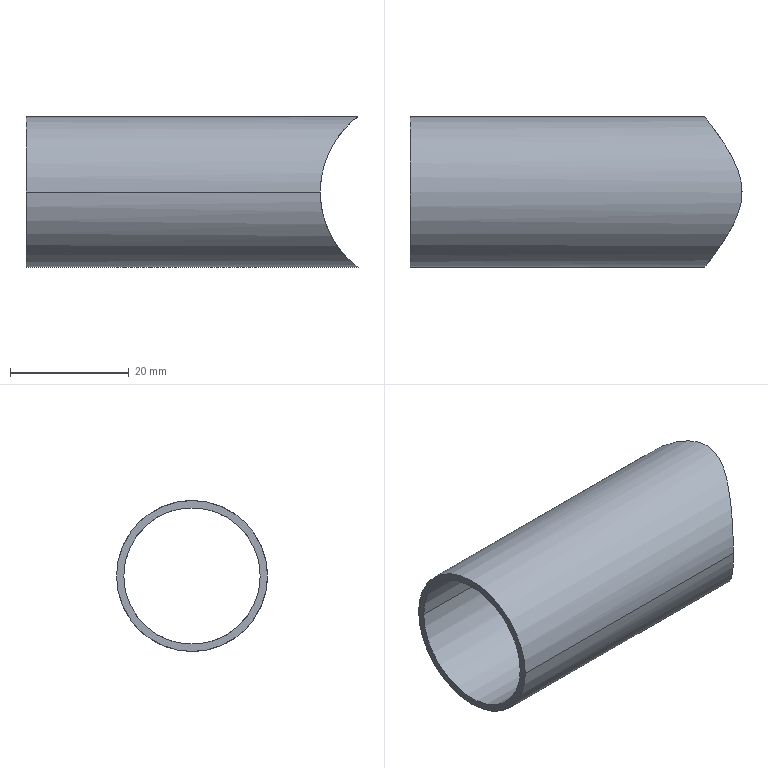Part | NX | features BREP 1 | 1 solid | 6 faces | box 55.88 x 25.4 x 25.4 mm | volume 4831 mm3 | cylinder 5 | plane 1 | commonest cylinder face diameters 22.962 x2 25.4 x2 31.75 x1
STEP:
#1=CARTESIAN_POINT('',(0.,12.7,0.));
#2=VERTEX_POINT('',#1);
#3=CARTESIAN_POINT('',(0.,-12.7,0.));
#4=VERTEX_POINT('',#3);
#5=CARTESIAN_POINT('',(0.,0.,0.));
#6=DIRECTION('',(1.,0.,0.));
#7=DIRECTION('',(0.,1.,0.));
#8=AXIS2_PLACEMENT_3D('',#5,#6,#7);
#9=CIRCLE('',#8,12.7);
#10=EDGE_CURVE('',#2,#4,#9,.T.);
#11=ORIENTED_EDGE('',*,*,#10,.F.);
#12=CARTESIAN_POINT('',(0.,0.,0.));
#13=DIRECTION('',(1.,0.,0.));
#14=DIRECTION('',(0.,-1.,0.));
#15=AXIS2_PLACEMENT_3D('',#12,#13,#14);
#16=CIRCLE('',#15,12.7);
#17=EDGE_CURVE('',#4,#2,#16,.T.);
#18=ORIENTED_EDGE('',*,*,#17,.F.);
#19=EDGE_LOOP('',(#11,#18));
#20=FACE_BOUND('',#19,.T.);
#21=CARTESIAN_POINT('',(0.,11.481,0.));
#22=VERTEX_POINT('',#21);
#23=CARTESIAN_POINT('',(0.,-11.481,0.));
#24=VERTEX_POINT('',#23);
#25=CARTESIAN_POINT('',(0.,0.,0.));
#26=DIRECTION('',(-1.,0.,0.));
#27=DIRECTION('',(0.,1.,0.));
#28=AXIS2_PLACEMENT_3D('',#25,#26,#27);
#29=CIRCLE('',#28,11.481);
#30=EDGE_CURVE('',#22,#24,#29,.T.);
#31=ORIENTED_EDGE('',*,*,#30,.F.);
#32=CARTESIAN_POINT('',(0.,0.,0.));
#33=DIRECTION('',(-1.,0.,0.));
#34=DIRECTION('',(0.,-1.,0.));
#35=AXIS2_PLACEMENT_3D('',#32,#33,#34);
#36=CIRCLE('',#35,11.481);
#37=EDGE_CURVE('',#24,#22,#36,.T.);
#38=ORIENTED_EDGE('',*,*,#37,.F.);
#39=EDGE_LOOP('',(#31,#38));
#40=FACE_BOUND('',#39,.T.);
#41=CARTESIAN_POINT('',(0.,0.,0.));
#42=DIRECTION('',(1.,0.,0.));
#43=DIRECTION('',(0.,1.,0.));
#44=AXIS2_PLACEMENT_3D('',#41,#42,#43);
#45=PLANE('',#44);
#46=ADVANCED_FACE('',(#20,#40),#45,.F.);
#47=CARTESIAN_POINT('',(49.53,-12.7,0.));
#48=VERTEX_POINT('',#47);
#49=CARTESIAN_POINT('',(0.,-12.7,0.));
#50=DIRECTION('',(1.,0.,0.));
#51=VECTOR('',#50,1000.);
#52=LINE('',#49,#51);
#53=EDGE_CURVE('',#4,#48,#52,.T.);
#54=ORIENTED_EDGE('',*,*,#53,.F.);
#55=ORIENTED_EDGE('',*,*,#17,.T.);
#56=CARTESIAN_POINT('',(49.53,12.7,0.));
#57=VERTEX_POINT('',#56);
#58=CARTESIAN_POINT('',(0.,12.7,0.));
#59=DIRECTION('',(1.,0.,0.));
#60=VECTOR('',#59,1000.);
#61=LINE('',#58,#60);
#62=EDGE_CURVE('',#2,#57,#61,.T.);
#63=ORIENTED_EDGE('',*,*,#62,.T.);
#64=CARTESIAN_POINT('',(49.53,12.7,0.));
#65=CARTESIAN_POINT('',(49.53,12.7,-0.9043));
#66=CARTESIAN_POINT('',(49.654,12.55,-2.294));
#67=CARTESIAN_POINT('',(50.047,12.051,-4.101));
#68=CARTESIAN_POINT('',(50.494,11.474,-5.502));
#69=CARTESIAN_POINT('',(50.866,10.987,-6.392));
#70=CARTESIAN_POINT('',(51.22,10.513,-7.139));
#71=CARTESIAN_POINT('',(51.549,10.063,-7.756));
#72=CARTESIAN_POINT('',(51.75,9.786,-8.099));
#73=CARTESIAN_POINT('',(52.106,9.286,-8.682));
#74=CARTESIAN_POINT('',(52.652,8.492,-9.472));
#75=CARTESIAN_POINT('',(53.22,7.601,-10.194));
#76=CARTESIAN_POINT('',(53.808,6.634,-10.854));
#77=CARTESIAN_POINT('',(54.417,5.517,-11.46));
#78=CARTESIAN_POINT('',(54.908,4.45,-11.915));
#79=CARTESIAN_POINT('',(55.357,3.259,-12.294));
#80=CARTESIAN_POINT('',(55.746,1.842,-12.601));
#81=CARTESIAN_POINT('',(55.972,-0.00789,-12.768));
#82=CARTESIAN_POINT('',(55.74,-1.867,-12.595));
#83=CARTESIAN_POINT('',(55.355,-3.266,-12.294));
#84=CARTESIAN_POINT('',(54.886,-4.499,-11.893));
#85=CARTESIAN_POINT('',(54.468,-5.399,-11.517));
#86=CARTESIAN_POINT('',(53.784,-6.679,-10.83));
#87=CARTESIAN_POINT('',(53.235,-7.593,-10.199));
#88=CARTESIAN_POINT('',(52.634,-8.518,-9.447));
#89=CARTESIAN_POINT('',(52.038,-9.374,-8.596));
#90=CARTESIAN_POINT('',(51.594,-10.003,-7.843));
#91=CARTESIAN_POINT('',(51.231,-10.498,-7.159));
#92=CARTESIAN_POINT('',(50.859,-10.997,-6.379));
#93=CARTESIAN_POINT('',(50.496,-11.471,-5.506));
#94=CARTESIAN_POINT('',(50.046,-12.052,-4.099));
#95=CARTESIAN_POINT('',(49.654,-12.55,-2.295));
#96=CARTESIAN_POINT('',(49.53,-12.7,-0.9044));
#97=CARTESIAN_POINT('',(49.53,-12.7,0.));
#98=B_SPLINE_CURVE_WITH_KNOTS('',3,(#64,#65,#66,#67,#68,#69,#70,#71,#72,#73,#74,#75,#76,#77,#78,#79,#80,#81,#82,#83,#84,#85,#86,#87,#88,#89,#90,#91,#92,#93,#94,#95,#96,#97),.UNSPECIFIED.,.F.,.F.,(4,1,1,1,1,1,1,1,1,1,1,1,1,1,1,1,1,1,1,1,1,1,1,1,1,1,1,1,1,1,1,4),(0.,0.0625,0.09375,0.125,0.1562,0.1719,0.1875,0.2031,0.2188,0.25,0.2812,0.3125,0.3438,0.375,0.4062,0.4375,0.5,0.5625,0.5938,0.625,0.6562,0.6875,0.7188,0.75,0.7812,0.8125,0.8281,0.8438,0.875,0.9062,0.9375,1.),.UNSPECIFIED.);
#99=EDGE_CURVE('',#57,#48,#98,.T.);
#100=ORIENTED_EDGE('',*,*,#99,.T.);
#101=EDGE_LOOP('',(#54,#55,#63,#100));
#102=FACE_BOUND('',#101,.T.);
#103=CARTESIAN_POINT('',(0.,0.,0.));
#104=DIRECTION('',(1.,0.,0.));
#105=DIRECTION('',(0.,-1.,0.));
#106=AXIS2_PLACEMENT_3D('',#103,#104,#105);
#107=CYLINDRICAL_SURFACE('',#106,12.7);
#108=ADVANCED_FACE('',(#102),#107,.T.);
#109=CARTESIAN_POINT('',(49.53,12.7,0.));
#110=CARTESIAN_POINT('',(49.53,12.7,0.9408));
#111=CARTESIAN_POINT('',(49.658,12.542,2.35));
#112=CARTESIAN_POINT('',(50.06,12.033,4.151));
#113=CARTESIAN_POINT('',(50.5,11.466,5.516));
#114=CARTESIAN_POINT('',(50.963,10.86,6.631));
#115=CARTESIAN_POINT('',(51.554,10.061,7.786));
#116=CARTESIAN_POINT('',(52.071,9.337,8.632));
#117=CARTESIAN_POINT('',(52.642,8.504,9.459));
#118=CARTESIAN_POINT('',(53.244,7.573,10.217));
#119=CARTESIAN_POINT('',(53.807,6.636,10.851));
#120=CARTESIAN_POINT('',(54.406,5.529,11.456));
#121=CARTESIAN_POINT('',(55.075,4.091,12.066));
#122=CARTESIAN_POINT('',(55.712,2.197,12.577));
#123=CARTESIAN_POINT('',(55.963,0.01076,12.76));
#124=CARTESIAN_POINT('',(55.716,-2.18,12.581));
#125=CARTESIAN_POINT('',(55.081,-4.075,12.072));
#126=CARTESIAN_POINT('',(54.412,-5.516,11.462));
#127=CARTESIAN_POINT('',(53.812,-6.626,10.856));
#128=CARTESIAN_POINT('',(53.248,-7.565,10.223));
#129=CARTESIAN_POINT('',(52.645,-8.5,9.463));
#130=CARTESIAN_POINT('',(52.073,-9.334,8.636));
#131=CARTESIAN_POINT('',(51.555,-10.059,7.788));
#132=CARTESIAN_POINT('',(50.964,-10.859,6.633));
#133=CARTESIAN_POINT('',(50.5,-11.466,5.517));
#134=CARTESIAN_POINT('',(50.06,-12.033,4.152));
#135=CARTESIAN_POINT('',(49.658,-12.542,2.351));
#136=CARTESIAN_POINT('',(49.53,-12.7,0.9409));
#137=CARTESIAN_POINT('',(49.53,-12.7,0.));
#138=B_SPLINE_CURVE_WITH_KNOTS('',3,(#109,#110,#111,#112,#113,#114,#115,#116,#117,#118,#119,#120,#121,#122,#123,#124,#125,#126,#127,#128,#129,#130,#131,#132,#133,#134,#135,#136,#137),.UNSPECIFIED.,.F.,.F.,(4,1,1,1,1,1,1,1,1,1,1,1,1,1,1,1,1,1,1,1,1,1,1,1,1,1,4),(0.,0.0625,0.09375,0.125,0.1562,0.1875,0.2188,0.25,0.2812,0.3125,0.3438,0.375,0.4375,0.5,0.5625,0.625,0.6562,0.6875,0.7188,0.75,0.7812,0.8125,0.8438,0.875,0.9062,0.9375,1.),.UNSPECIFIED.);
#139=EDGE_CURVE('',#48,#57,#138,.F.);
#140=ORIENTED_EDGE('',*,*,#139,.F.);
#141=ORIENTED_EDGE('',*,*,#99,.F.);
#142=EDGE_LOOP('',(#140,#141));
#143=FACE_BOUND('',#142,.T.);
#144=CARTESIAN_POINT('',(49.53,11.481,0.));
#145=VERTEX_POINT('',#144);
#146=CARTESIAN_POINT('',(49.53,-11.481,0.));
#147=VERTEX_POINT('',#146);
#148=CARTESIAN_POINT('',(49.53,-11.481,0.));
#149=CARTESIAN_POINT('',(49.53,-11.481,1.476));
#150=CARTESIAN_POINT('',(49.83,-11.074,3.639));
#151=CARTESIAN_POINT('',(50.823,-9.633,6.391));
#152=CARTESIAN_POINT('',(51.731,-8.203,8.143));
#153=CARTESIAN_POINT('',(52.811,-6.291,9.717));
#154=CARTESIAN_POINT('',(53.77,-4.059,10.818));
#155=CARTESIAN_POINT('',(54.307,-2.064,11.354));
#156=CARTESIAN_POINT('',(54.508,0.001942,11.545));
#157=CARTESIAN_POINT('',(54.307,2.067,11.354));
#158=CARTESIAN_POINT('',(53.769,4.063,10.817));
#159=CARTESIAN_POINT('',(52.809,6.296,9.714));
#160=CARTESIAN_POINT('',(51.73,8.206,8.14));
#161=CARTESIAN_POINT('',(50.823,9.634,6.389));
#162=CARTESIAN_POINT('',(49.83,11.073,3.639));
#163=CARTESIAN_POINT('',(49.53,11.481,1.476));
#164=CARTESIAN_POINT('',(49.53,11.481,0.));
#165=B_SPLINE_CURVE_WITH_KNOTS('',3,(#148,#149,#150,#151,#152,#153,#154,#155,#156,#157,#158,#159,#160,#161,#162,#163,#164),.UNSPECIFIED.,.F.,.F.,(4,1,1,1,1,1,1,1,1,1,1,1,1,1,4),(0.,0.125,0.1875,0.25,0.3125,0.375,0.4375,0.5,0.5625,0.625,0.6875,0.75,0.8125,0.875,1.),.UNSPECIFIED.);
#166=EDGE_CURVE('',#145,#147,#165,.F.);
#167=ORIENTED_EDGE('',*,*,#166,.F.);
#168=CARTESIAN_POINT('',(49.53,11.481,0.));
#169=CARTESIAN_POINT('',(49.53,11.481,-1.475));
#170=CARTESIAN_POINT('',(49.83,11.074,-3.637));
#171=CARTESIAN_POINT('',(50.823,9.634,-6.39));
#172=CARTESIAN_POINT('',(51.731,8.204,-8.142));
#173=CARTESIAN_POINT('',(52.811,6.291,-9.718));
#174=CARTESIAN_POINT('',(53.77,4.06,-10.818));
#175=CARTESIAN_POINT('',(54.307,2.065,-11.354));
#176=CARTESIAN_POINT('',(54.508,-0.00009445,-11.544));
#177=CARTESIAN_POINT('',(54.307,-2.064,-11.354));
#178=CARTESIAN_POINT('',(53.77,-4.059,-10.818));
#179=CARTESIAN_POINT('',(52.811,-6.291,-9.718));
#180=CARTESIAN_POINT('',(51.731,-8.205,-8.142));
#181=CARTESIAN_POINT('',(50.823,-9.634,-6.39));
#182=CARTESIAN_POINT('',(49.83,-11.074,-3.636));
#183=CARTESIAN_POINT('',(49.53,-11.481,-1.475));
#184=CARTESIAN_POINT('',(49.53,-11.481,0.));
#185=B_SPLINE_CURVE_WITH_KNOTS('',3,(#168,#169,#170,#171,#172,#173,#174,#175,#176,#177,#178,#179,#180,#181,#182,#183,#184),.UNSPECIFIED.,.F.,.F.,(4,1,1,1,1,1,1,1,1,1,1,1,1,1,4),(0.,0.125,0.1875,0.25,0.3125,0.375,0.4375,0.5,0.5625,0.625,0.6875,0.75,0.8125,0.875,1.),.UNSPECIFIED.);
#186=EDGE_CURVE('',#147,#145,#185,.F.);
#187=ORIENTED_EDGE('',*,*,#186,.F.);
#188=EDGE_LOOP('',(#167,#187));
#189=FACE_BOUND('',#188,.T.);
#190=CARTESIAN_POINT('',(65.405,15.24,0.));
#191=DIRECTION('',(0.,1.,0.));
#192=DIRECTION('',(1.,0.,0.));
#193=AXIS2_PLACEMENT_3D('',#190,#191,#192);
#194=CYLINDRICAL_SURFACE('',#193,15.875);
#195=ADVANCED_FACE('',(#143,#189),#194,.F.);
#196=ORIENTED_EDGE('',*,*,#62,.F.);
#197=ORIENTED_EDGE('',*,*,#10,.T.);
#198=ORIENTED_EDGE('',*,*,#53,.T.);
#199=ORIENTED_EDGE('',*,*,#139,.T.);
#200=EDGE_LOOP('',(#196,#197,#198,#199));
#201=FACE_BOUND('',#200,.T.);
#202=CARTESIAN_POINT('',(0.,0.,0.));
#203=DIRECTION('',(1.,0.,0.));
#204=DIRECTION('',(0.,-1.,0.));
#205=AXIS2_PLACEMENT_3D('',#202,#203,#204);
#206=CYLINDRICAL_SURFACE('',#205,12.7);
#207=ADVANCED_FACE('',(#201),#206,.T.);
#208=CARTESIAN_POINT('',(0.,11.481,0.));
#209=DIRECTION('',(1.,0.,0.));
#210=VECTOR('',#209,1000.);
#211=LINE('',#208,#210);
#212=EDGE_CURVE('',#145,#22,#211,.F.);
#213=ORIENTED_EDGE('',*,*,#212,.T.);
#214=ORIENTED_EDGE('',*,*,#30,.T.);
#215=CARTESIAN_POINT('',(0.,-11.481,0.));
#216=DIRECTION('',(1.,0.,0.));
#217=VECTOR('',#216,1000.);
#218=LINE('',#215,#217);
#219=EDGE_CURVE('',#147,#24,#218,.F.);
#220=ORIENTED_EDGE('',*,*,#219,.F.);
#221=ORIENTED_EDGE('',*,*,#186,.T.);
#222=EDGE_LOOP('',(#213,#214,#220,#221));
#223=FACE_BOUND('',#222,.T.);
#224=CARTESIAN_POINT('',(0.,0.,0.));
#225=DIRECTION('',(1.,0.,0.));
#226=DIRECTION('',(0.,-1.,0.));
#227=AXIS2_PLACEMENT_3D('',#224,#225,#226);
#228=CYLINDRICAL_SURFACE('',#227,11.481);
#229=ADVANCED_FACE('',(#223),#228,.F.);
#230=ORIENTED_EDGE('',*,*,#219,.T.);
#231=ORIENTED_EDGE('',*,*,#37,.T.);
#232=ORIENTED_EDGE('',*,*,#212,.F.);
#233=ORIENTED_EDGE('',*,*,#166,.T.);
#234=EDGE_LOOP('',(#230,#231,#232,#233));
#235=FACE_BOUND('',#234,.T.);
#236=CARTESIAN_POINT('',(0.,0.,0.));
#237=DIRECTION('',(1.,0.,0.));
#238=DIRECTION('',(0.,-1.,0.));
#239=AXIS2_PLACEMENT_3D('',#236,#237,#238);
#240=CYLINDRICAL_SURFACE('',#239,11.481);
#241=ADVANCED_FACE('',(#235),#240,.F.);
#242=CLOSED_SHELL('',(#46,#108,#195,#207,#229,#241));
#243=MANIFOLD_SOLID_BREP('',#242);
#244=(LENGTH_UNIT()NAMED_UNIT(*)SI_UNIT(.MILLI.,.METRE.));
#245=UNCERTAINTY_MEASURE_WITH_UNIT(LENGTH_MEASURE(0.0508),#244,'','');
#246=(NAMED_UNIT(*)PLANE_ANGLE_UNIT()SI_UNIT($,.RADIAN.));
#247=(NAMED_UNIT(*)SI_UNIT($,.STERADIAN.)SOLID_ANGLE_UNIT());
#248=(GEOMETRIC_REPRESENTATION_CONTEXT(3)GLOBAL_UNCERTAINTY_ASSIGNED_CONTEXT((#245))GLOBAL_UNIT_ASSIGNED_CONTEXT((#244,#246,#247))REPRESENTATION_CONTEXT('',''));
#249=ADVANCED_BREP_SHAPE_REPRESENTATION('',(#243),#248);